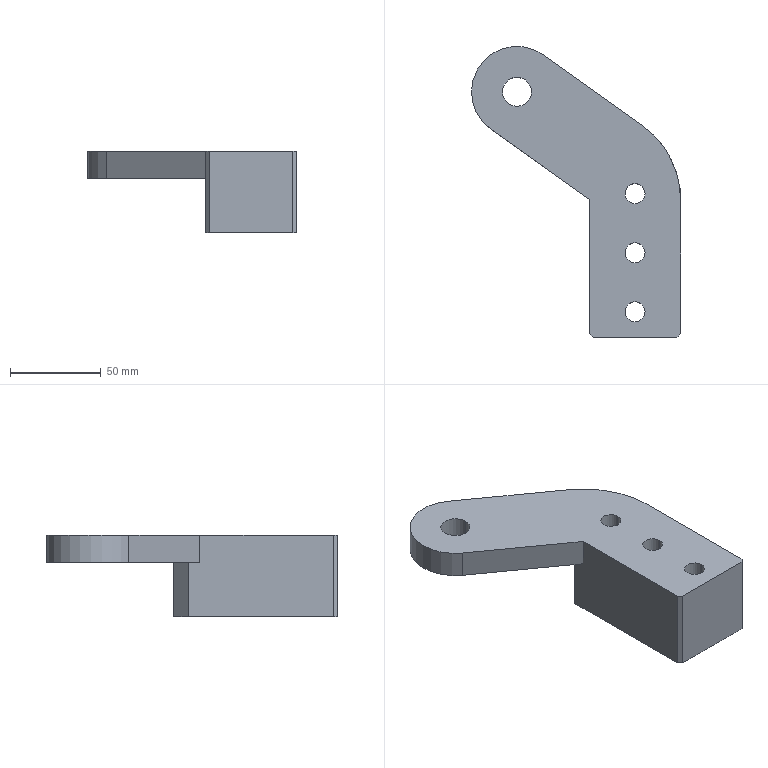Part | Creo | features DATUM PLANE 3, CURVE 2, PROTRUSION 2, CHAMFER 1, COORDINATE SYSTEM 1 | 1 solid | 24 faces | box 115 x 160.005 x 45 mm | volume 256646 mm3 | plane 14 | cylinder 10 | commonest cylinder face diameters 11 x6 16 x2 50 x1 100 x1
STEP:
#1=CARTESIAN_POINT('',(0.,0.,0.));
#2=DIRECTION('',(0.,0.,1.));
#3=DIRECTION('',(1.,0.,0.));
#4=AXIS2_PLACEMENT_3D('',#1,#2,#3);
#5=CARTESIAN_POINT('',(-25.,75.708,0.));
#6=VERTEX_POINT('',#5);
#7=CARTESIAN_POINT('',(-25.,82.,0.));
#8=VERTEX_POINT('',#7);
#9=CARTESIAN_POINT('',(-25.,75.708,0.));
#10=DIRECTION('',(0.,1.,0.));
#11=VECTOR('',#10,6.292);
#12=LINE('',#9,#11);
#13=EDGE_CURVE('',#6,#8,#12,.T.);
#14=ORIENTED_EDGE('',*,*,#13,.T.);
#15=CARTESIAN_POINT('',(-17.,90.,0.));
#16=VERTEX_POINT('',#15);
#17=CARTESIAN_POINT('',(-17.,90.,0.));
#18=DIRECTION('',(-0.7071,-0.7071,0.));
#19=VECTOR('',#18,11.314);
#20=LINE('',#17,#19);
#21=EDGE_CURVE('',#16,#8,#20,.T.);
#22=ORIENTED_EDGE('',*,*,#21,.F.);
#23=CARTESIAN_POINT('',(17.,90.,0.));
#24=VERTEX_POINT('',#23);
#25=CARTESIAN_POINT('',(17.,90.,0.));
#26=DIRECTION('',(-1.,0.,0.));
#27=VECTOR('',#26,34.);
#28=LINE('',#25,#27);
#29=EDGE_CURVE('',#24,#16,#28,.T.);
#30=ORIENTED_EDGE('',*,*,#29,.F.);
#31=CARTESIAN_POINT('',(24.542,82.458,0.));
#32=VERTEX_POINT('',#31);
#33=CARTESIAN_POINT('',(24.542,82.458,0.));
#34=DIRECTION('',(-0.7071,0.7071,0.));
#35=VECTOR('',#34,10.666);
#36=LINE('',#33,#35);
#37=EDGE_CURVE('',#32,#24,#36,.T.);
#38=ORIENTED_EDGE('',*,*,#37,.F.);
#39=CARTESIAN_POINT('',(4.064,116.393,0.));
#40=VERTEX_POINT('',#39);
#41=CARTESIAN_POINT('',(-25.,75.708,0.));
#42=DIRECTION('',(0.,0.,1.));
#43=DIRECTION('',(0.9908,0.135,0.));
#44=AXIS2_PLACEMENT_3D('',#41,#42,#43);
#45=CIRCLE('',#44,50.);
#46=EDGE_CURVE('',#32,#40,#45,.T.);
#47=ORIENTED_EDGE('',*,*,#46,.T.);
#48=CARTESIAN_POINT('',(-50.468,155.348,0.));
#49=VERTEX_POINT('',#48);
#50=CARTESIAN_POINT('',(4.064,116.393,0.));
#51=DIRECTION('',(-0.8137,0.5813,0.));
#52=VECTOR('',#51,67.016);
#53=LINE('',#50,#52);
#54=EDGE_CURVE('',#40,#49,#53,.T.);
#55=ORIENTED_EDGE('',*,*,#54,.T.);
#56=CARTESIAN_POINT('',(-79.532,114.662,0.));
#57=VERTEX_POINT('',#56);
#58=CARTESIAN_POINT('',(-65.,135.005,0.));
#59=DIRECTION('',(0.,0.,1.));
#60=DIRECTION('',(0.5813,0.8137,0.));
#61=AXIS2_PLACEMENT_3D('',#58,#59,#60);
#62=CIRCLE('',#61,25.);
#63=EDGE_CURVE('',#49,#57,#62,.T.);
#64=ORIENTED_EDGE('',*,*,#63,.T.);
#65=CARTESIAN_POINT('',(-79.532,114.662,0.));
#66=DIRECTION('',(0.8137,-0.5813,0.));
#67=VECTOR('',#66,67.016);
#68=LINE('',#65,#67);
#69=EDGE_CURVE('',#57,#6,#68,.T.);
#70=ORIENTED_EDGE('',*,*,#69,.T.);
#71=EDGE_LOOP('',(#14,#22,#30,#38,#47,#55,#64,#70));
#72=FACE_OUTER_BOUND('',#71,.F.);
#73=CARTESIAN_POINT('',(-57.,135.005,0.));
#74=VERTEX_POINT('',#73);
#75=CARTESIAN_POINT('',(-73.,135.005,0.));
#76=VERTEX_POINT('',#75);
#77=CARTESIAN_POINT('',(-65.,135.005,0.));
#78=DIRECTION('',(0.,0.,-1.));
#79=DIRECTION('',(1.,0.,0.));
#80=AXIS2_PLACEMENT_3D('',#77,#78,#79);
#81=CIRCLE('',#80,8.);
#82=EDGE_CURVE('',#74,#76,#81,.T.);
#83=ORIENTED_EDGE('',*,*,#82,.T.);
#84=CARTESIAN_POINT('',(-65.,135.005,0.));
#85=DIRECTION('',(0.,0.,-1.));
#86=DIRECTION('',(-1.,0.,0.));
#87=AXIS2_PLACEMENT_3D('',#84,#85,#86);
#88=CIRCLE('',#87,8.);
#89=EDGE_CURVE('',#76,#74,#88,.T.);
#90=ORIENTED_EDGE('',*,*,#89,.T.);
#91=EDGE_LOOP('',(#83,#90));
#92=FACE_BOUND('',#91,.F.);
#93=CARTESIAN_POINT('',(0.,0.,0.));
#94=DIRECTION('',(0.,0.,1.));
#95=DIRECTION('',(1.,0.,0.));
#96=AXIS2_PLACEMENT_3D('',#93,#94,#95);
#97=PLANE('',#96);
#98=ADVANCED_FACE('',(#72,#92),#97,.F.);
#99=ORIENTED_EDGE('',*,*,#82,.F.);
#100=CARTESIAN_POINT('',(-57.,135.005,15.));
#101=VERTEX_POINT('',#100);
#102=CARTESIAN_POINT('',(-57.,135.005,0.));
#103=DIRECTION('',(0.,0.,1.));
#104=VECTOR('',#103,15.);
#105=LINE('',#102,#104);
#106=EDGE_CURVE('',#74,#101,#105,.T.);
#107=ORIENTED_EDGE('',*,*,#106,.T.);
#108=CARTESIAN_POINT('',(-73.,135.005,15.));
#109=VERTEX_POINT('',#108);
#110=CARTESIAN_POINT('',(-65.,135.005,15.));
#111=DIRECTION('',(0.,0.,-1.));
#112=DIRECTION('',(1.,0.,0.));
#113=AXIS2_PLACEMENT_3D('',#110,#111,#112);
#114=CIRCLE('',#113,8.);
#115=EDGE_CURVE('',#101,#109,#114,.T.);
#116=ORIENTED_EDGE('',*,*,#115,.T.);
#117=CARTESIAN_POINT('',(-73.,135.005,0.));
#118=DIRECTION('',(0.,0.,1.));
#119=VECTOR('',#118,15.);
#120=LINE('',#117,#119);
#121=EDGE_CURVE('',#76,#109,#120,.T.);
#122=ORIENTED_EDGE('',*,*,#121,.F.);
#123=EDGE_LOOP('',(#99,#107,#116,#122));
#124=FACE_OUTER_BOUND('',#123,.F.);
#125=CARTESIAN_POINT('',(-65.,135.005,0.));
#126=DIRECTION('',(0.,0.,1.));
#127=DIRECTION('',(1.,0.,0.));
#128=AXIS2_PLACEMENT_3D('',#125,#126,#127);
#129=CYLINDRICAL_SURFACE('',#128,8.);
#130=ADVANCED_FACE('',(#124),#129,.F.);
#131=ORIENTED_EDGE('',*,*,#89,.F.);
#132=ORIENTED_EDGE('',*,*,#121,.T.);
#133=CARTESIAN_POINT('',(-65.,135.005,15.));
#134=DIRECTION('',(0.,0.,-1.));
#135=DIRECTION('',(-1.,0.,0.));
#136=AXIS2_PLACEMENT_3D('',#133,#134,#135);
#137=CIRCLE('',#136,8.);
#138=EDGE_CURVE('',#109,#101,#137,.T.);
#139=ORIENTED_EDGE('',*,*,#138,.T.);
#140=ORIENTED_EDGE('',*,*,#106,.F.);
#141=EDGE_LOOP('',(#131,#132,#139,#140));
#142=FACE_OUTER_BOUND('',#141,.F.);
#143=CARTESIAN_POINT('',(-65.,135.005,0.));
#144=DIRECTION('',(0.,0.,1.));
#145=DIRECTION('',(1.,0.,0.));
#146=AXIS2_PLACEMENT_3D('',#143,#144,#145);
#147=CYLINDRICAL_SURFACE('',#146,8.);
#148=ADVANCED_FACE('',(#142),#147,.F.);
#149=CARTESIAN_POINT('',(-23.,0.,15.));
#150=VERTEX_POINT('',#149);
#151=CARTESIAN_POINT('',(23.,0.,15.));
#152=VERTEX_POINT('',#151);
#153=CARTESIAN_POINT('',(-23.,0.,15.));
#154=DIRECTION('',(1.,0.,0.));
#155=VECTOR('',#154,46.);
#156=LINE('',#153,#155);
#157=EDGE_CURVE('',#150,#152,#156,.T.);
#158=ORIENTED_EDGE('',*,*,#157,.F.);
#159=CARTESIAN_POINT('',(-25.,2.,15.));
#160=VERTEX_POINT('',#159);
#161=CARTESIAN_POINT('',(-25.,2.,15.));
#162=DIRECTION('',(0.7071,-0.7071,0.));
#163=VECTOR('',#162,2.828);
#164=LINE('',#161,#163);
#165=EDGE_CURVE('',#160,#150,#164,.T.);
#166=ORIENTED_EDGE('',*,*,#165,.F.);
#167=CARTESIAN_POINT('',(-25.,75.708,15.));
#168=VERTEX_POINT('',#167);
#169=CARTESIAN_POINT('',(-25.,75.708,15.));
#170=DIRECTION('',(0.,-1.,0.));
#171=VECTOR('',#170,73.708);
#172=LINE('',#169,#171);
#173=EDGE_CURVE('',#168,#160,#172,.T.);
#174=ORIENTED_EDGE('',*,*,#173,.F.);
#175=CARTESIAN_POINT('',(-79.532,114.662,15.));
#176=VERTEX_POINT('',#175);
#177=CARTESIAN_POINT('',(-79.532,114.662,15.));
#178=DIRECTION('',(0.8137,-0.5813,0.));
#179=VECTOR('',#178,67.016);
#180=LINE('',#177,#179);
#181=EDGE_CURVE('',#176,#168,#180,.T.);
#182=ORIENTED_EDGE('',*,*,#181,.F.);
#183=CARTESIAN_POINT('',(-50.468,155.348,15.));
#184=VERTEX_POINT('',#183);
#185=CARTESIAN_POINT('',(-65.,135.005,15.));
#186=DIRECTION('',(0.,0.,1.));
#187=DIRECTION('',(0.5813,0.8137,0.));
#188=AXIS2_PLACEMENT_3D('',#185,#186,#187);
#189=CIRCLE('',#188,25.);
#190=EDGE_CURVE('',#184,#176,#189,.T.);
#191=ORIENTED_EDGE('',*,*,#190,.F.);
#192=CARTESIAN_POINT('',(4.064,116.393,15.));
#193=VERTEX_POINT('',#192);
#194=CARTESIAN_POINT('',(4.064,116.393,15.));
#195=DIRECTION('',(-0.8137,0.5813,0.));
#196=VECTOR('',#195,67.016);
#197=LINE('',#194,#196);
#198=EDGE_CURVE('',#193,#184,#197,.T.);
#199=ORIENTED_EDGE('',*,*,#198,.F.);
#200=CARTESIAN_POINT('',(25.,75.708,15.));
#201=VERTEX_POINT('',#200);
#202=CARTESIAN_POINT('',(-25.,75.708,15.));
#203=DIRECTION('',(0.,0.,1.));
#204=DIRECTION('',(1.,0.,0.));
#205=AXIS2_PLACEMENT_3D('',#202,#203,#204);
#206=CIRCLE('',#205,50.);
#207=EDGE_CURVE('',#201,#193,#206,.T.);
#208=ORIENTED_EDGE('',*,*,#207,.F.);
#209=CARTESIAN_POINT('',(25.,2.,15.));
#210=VERTEX_POINT('',#209);
#211=CARTESIAN_POINT('',(25.,2.,15.));
#212=DIRECTION('',(0.,1.,0.));
#213=VECTOR('',#212,73.708);
#214=LINE('',#211,#213);
#215=EDGE_CURVE('',#210,#201,#214,.T.);
#216=ORIENTED_EDGE('',*,*,#215,.F.);
#217=CARTESIAN_POINT('',(23.,0.,15.));
#218=DIRECTION('',(0.7071,0.7071,0.));
#219=VECTOR('',#218,2.828);
#220=LINE('',#217,#219);
#221=EDGE_CURVE('',#152,#210,#220,.T.);
#222=ORIENTED_EDGE('',*,*,#221,.F.);
#223=EDGE_LOOP('',(#158,#166,#174,#182,#191,#199,#208,#216,#222));
#224=FACE_OUTER_BOUND('',#223,.F.);
#225=CARTESIAN_POINT('',(5.5,79.,15.));
#226=VERTEX_POINT('',#225);
#227=CARTESIAN_POINT('',(-5.5,79.,15.));
#228=VERTEX_POINT('',#227);
#229=CARTESIAN_POINT('',(0.,79.,15.));
#230=DIRECTION('',(0.,0.,-1.));
#231=DIRECTION('',(1.,0.,0.));
#232=AXIS2_PLACEMENT_3D('',#229,#230,#231);
#233=CIRCLE('',#232,5.5);
#234=EDGE_CURVE('',#226,#228,#233,.T.);
#235=ORIENTED_EDGE('',*,*,#234,.F.);
#236=CARTESIAN_POINT('',(0.,79.,15.));
#237=DIRECTION('',(0.,0.,-1.));
#238=DIRECTION('',(-1.,0.,0.));
#239=AXIS2_PLACEMENT_3D('',#236,#237,#238);
#240=CIRCLE('',#239,5.5);
#241=EDGE_CURVE('',#228,#226,#240,.T.);
#242=ORIENTED_EDGE('',*,*,#241,.F.);
#243=EDGE_LOOP('',(#235,#242));
#244=FACE_BOUND('',#243,.F.);
#245=CARTESIAN_POINT('',(5.5,46.5,15.));
#246=VERTEX_POINT('',#245);
#247=CARTESIAN_POINT('',(-5.5,46.5,15.));
#248=VERTEX_POINT('',#247);
#249=CARTESIAN_POINT('',(0.,46.5,15.));
#250=DIRECTION('',(0.,0.,-1.));
#251=DIRECTION('',(1.,0.,0.));
#252=AXIS2_PLACEMENT_3D('',#249,#250,#251);
#253=CIRCLE('',#252,5.5);
#254=EDGE_CURVE('',#246,#248,#253,.T.);
#255=ORIENTED_EDGE('',*,*,#254,.F.);
#256=CARTESIAN_POINT('',(0.,46.5,15.));
#257=DIRECTION('',(0.,0.,-1.));
#258=DIRECTION('',(-1.,0.,0.));
#259=AXIS2_PLACEMENT_3D('',#256,#257,#258);
#260=CIRCLE('',#259,5.5);
#261=EDGE_CURVE('',#248,#246,#260,.T.);
#262=ORIENTED_EDGE('',*,*,#261,.F.);
#263=EDGE_LOOP('',(#255,#262));
#264=FACE_BOUND('',#263,.F.);
#265=ORIENTED_EDGE('',*,*,#115,.F.);
#266=ORIENTED_EDGE('',*,*,#138,.F.);
#267=EDGE_LOOP('',(#265,#266));
#268=FACE_BOUND('',#267,.F.);
#269=CARTESIAN_POINT('',(5.5,14.,15.));
#270=VERTEX_POINT('',#269);
#271=CARTESIAN_POINT('',(-5.5,14.,15.));
#272=VERTEX_POINT('',#271);
#273=CARTESIAN_POINT('',(0.,14.,15.));
#274=DIRECTION('',(0.,0.,-1.));
#275=DIRECTION('',(1.,0.,0.));
#276=AXIS2_PLACEMENT_3D('',#273,#274,#275);
#277=CIRCLE('',#276,5.5);
#278=EDGE_CURVE('',#270,#272,#277,.T.);
#279=ORIENTED_EDGE('',*,*,#278,.F.);
#280=CARTESIAN_POINT('',(0.,14.,15.));
#281=DIRECTION('',(0.,0.,-1.));
#282=DIRECTION('',(-1.,0.,0.));
#283=AXIS2_PLACEMENT_3D('',#280,#281,#282);
#284=CIRCLE('',#283,5.5);
#285=EDGE_CURVE('',#272,#270,#284,.T.);
#286=ORIENTED_EDGE('',*,*,#285,.F.);
#287=EDGE_LOOP('',(#279,#286));
#288=FACE_BOUND('',#287,.F.);
#289=CARTESIAN_POINT('',(0.,0.,15.));
#290=DIRECTION('',(0.,0.,1.));
#291=DIRECTION('',(1.,0.,0.));
#292=AXIS2_PLACEMENT_3D('',#289,#290,#291);
#293=PLANE('',#292);
#294=ADVANCED_FACE('',(#224,#244,#264,#268,#288),#293,.T.);
#295=CARTESIAN_POINT('',(-5.5,14.,-30.));
#296=VERTEX_POINT('',#295);
#297=CARTESIAN_POINT('',(-5.5,14.,15.));
#298=DIRECTION('',(0.,0.,-1.));
#299=VECTOR('',#298,45.);
#300=LINE('',#297,#299);
#301=EDGE_CURVE('',#272,#296,#300,.T.);
#302=ORIENTED_EDGE('',*,*,#301,.T.);
#303=CARTESIAN_POINT('',(5.5,14.,-30.));
#304=VERTEX_POINT('',#303);
#305=CARTESIAN_POINT('',(0.,14.,-30.));
#306=DIRECTION('',(0.,0.,1.));
#307=DIRECTION('',(-1.,0.,0.));
#308=AXIS2_PLACEMENT_3D('',#305,#306,#307);
#309=CIRCLE('',#308,5.5);
#310=EDGE_CURVE('',#296,#304,#309,.T.);
#311=ORIENTED_EDGE('',*,*,#310,.T.);
#312=CARTESIAN_POINT('',(5.5,14.,-30.));
#313=DIRECTION('',(0.,0.,1.));
#314=VECTOR('',#313,45.);
#315=LINE('',#312,#314);
#316=EDGE_CURVE('',#304,#270,#315,.T.);
#317=ORIENTED_EDGE('',*,*,#316,.T.);
#318=ORIENTED_EDGE('',*,*,#278,.T.);
#319=EDGE_LOOP('',(#302,#311,#317,#318));
#320=FACE_OUTER_BOUND('',#319,.F.);
#321=CARTESIAN_POINT('',(0.,14.,0.));
#322=DIRECTION('',(0.,0.,1.));
#323=DIRECTION('',(1.,0.,0.));
#324=AXIS2_PLACEMENT_3D('',#321,#322,#323);
#325=CYLINDRICAL_SURFACE('',#324,5.5);
#326=ADVANCED_FACE('',(#320),#325,.F.);
#327=ORIENTED_EDGE('',*,*,#316,.F.);
#328=CARTESIAN_POINT('',(0.,14.,-30.));
#329=DIRECTION('',(0.,0.,1.));
#330=DIRECTION('',(1.,0.,0.));
#331=AXIS2_PLACEMENT_3D('',#328,#329,#330);
#332=CIRCLE('',#331,5.5);
#333=EDGE_CURVE('',#304,#296,#332,.T.);
#334=ORIENTED_EDGE('',*,*,#333,.T.);
#335=ORIENTED_EDGE('',*,*,#301,.F.);
#336=ORIENTED_EDGE('',*,*,#285,.T.);
#337=EDGE_LOOP('',(#327,#334,#335,#336));
#338=FACE_OUTER_BOUND('',#337,.F.);
#339=CARTESIAN_POINT('',(0.,14.,0.));
#340=DIRECTION('',(0.,0.,1.));
#341=DIRECTION('',(1.,0.,0.));
#342=AXIS2_PLACEMENT_3D('',#339,#340,#341);
#343=CYLINDRICAL_SURFACE('',#342,5.5);
#344=ADVANCED_FACE('',(#338),#343,.F.);
#345=CARTESIAN_POINT('',(17.,90.,-30.));
#346=VERTEX_POINT('',#345);
#347=CARTESIAN_POINT('',(25.,82.,-30.));
#348=VERTEX_POINT('',#347);
#349=CARTESIAN_POINT('',(17.,90.,-30.));
#350=DIRECTION('',(0.7071,-0.7071,0.));
#351=VECTOR('',#350,11.314);
#352=LINE('',#349,#351);
#353=EDGE_CURVE('',#346,#348,#352,.T.);
#354=ORIENTED_EDGE('',*,*,#353,.F.);
#355=CARTESIAN_POINT('',(-17.,90.,-30.));
#356=VERTEX_POINT('',#355);
#357=CARTESIAN_POINT('',(-17.,90.,-30.));
#358=DIRECTION('',(1.,0.,0.));
#359=VECTOR('',#358,34.);
#360=LINE('',#357,#359);
#361=EDGE_CURVE('',#356,#346,#360,.T.);
#362=ORIENTED_EDGE('',*,*,#361,.F.);
#363=CARTESIAN_POINT('',(-25.,82.,-30.));
#364=VERTEX_POINT('',#363);
#365=CARTESIAN_POINT('',(-25.,82.,-30.));
#366=DIRECTION('',(0.7071,0.7071,0.));
#367=VECTOR('',#366,11.314);
#368=LINE('',#365,#367);
#369=EDGE_CURVE('',#364,#356,#368,.T.);
#370=ORIENTED_EDGE('',*,*,#369,.F.);
#371=CARTESIAN_POINT('',(-25.,2.,-30.));
#372=VERTEX_POINT('',#371);
#373=CARTESIAN_POINT('',(-25.,2.,-30.));
#374=DIRECTION('',(0.,1.,0.));
#375=VECTOR('',#374,80.);
#376=LINE('',#373,#375);
#377=EDGE_CURVE('',#372,#364,#376,.T.);
#378=ORIENTED_EDGE('',*,*,#377,.F.);
#379=CARTESIAN_POINT('',(-23.,0.,-30.));
#380=VERTEX_POINT('',#379);
#381=CARTESIAN_POINT('',(-23.,0.,-30.));
#382=DIRECTION('',(-0.7071,0.7071,0.));
#383=VECTOR('',#382,2.828);
#384=LINE('',#381,#383);
#385=EDGE_CURVE('',#380,#372,#384,.T.);
#386=ORIENTED_EDGE('',*,*,#385,.F.);
#387=CARTESIAN_POINT('',(23.,0.,-30.));
#388=VERTEX_POINT('',#387);
#389=CARTESIAN_POINT('',(23.,0.,-30.));
#390=DIRECTION('',(-1.,0.,0.));
#391=VECTOR('',#390,46.);
#392=LINE('',#389,#391);
#393=EDGE_CURVE('',#388,#380,#392,.T.);
#394=ORIENTED_EDGE('',*,*,#393,.F.);
#395=CARTESIAN_POINT('',(25.,2.,-30.));
#396=VERTEX_POINT('',#395);
#397=CARTESIAN_POINT('',(25.,2.,-30.));
#398=DIRECTION('',(-0.7071,-0.7071,0.));
#399=VECTOR('',#398,2.828);
#400=LINE('',#397,#399);
#401=EDGE_CURVE('',#396,#388,#400,.T.);
#402=ORIENTED_EDGE('',*,*,#401,.F.);
#403=CARTESIAN_POINT('',(25.,82.,-30.));
#404=DIRECTION('',(0.,-1.,0.));
#405=VECTOR('',#404,80.);
#406=LINE('',#403,#405);
#407=EDGE_CURVE('',#348,#396,#406,.T.);
#408=ORIENTED_EDGE('',*,*,#407,.F.);
#409=EDGE_LOOP('',(#354,#362,#370,#378,#386,#394,#402,#408));
#410=FACE_OUTER_BOUND('',#409,.F.);
#411=CARTESIAN_POINT('',(-5.5,46.5,-30.));
#412=VERTEX_POINT('',#411);
#413=CARTESIAN_POINT('',(5.5,46.5,-30.));
#414=VERTEX_POINT('',#413);
#415=CARTESIAN_POINT('',(0.,46.5,-30.));
#416=DIRECTION('',(0.,0.,1.));
#417=DIRECTION('',(-1.,0.,0.));
#418=AXIS2_PLACEMENT_3D('',#415,#416,#417);
#419=CIRCLE('',#418,5.5);
#420=EDGE_CURVE('',#412,#414,#419,.T.);
#421=ORIENTED_EDGE('',*,*,#420,.F.);
#422=CARTESIAN_POINT('',(0.,46.5,-30.));
#423=DIRECTION('',(0.,0.,1.));
#424=DIRECTION('',(1.,0.,0.));
#425=AXIS2_PLACEMENT_3D('',#422,#423,#424);
#426=CIRCLE('',#425,5.5);
#427=EDGE_CURVE('',#414,#412,#426,.T.);
#428=ORIENTED_EDGE('',*,*,#427,.F.);
#429=EDGE_LOOP('',(#421,#428));
#430=FACE_BOUND('',#429,.F.);
#431=ORIENTED_EDGE('',*,*,#333,.F.);
#432=ORIENTED_EDGE('',*,*,#310,.F.);
#433=EDGE_LOOP('',(#431,#432));
#434=FACE_BOUND('',#433,.F.);
#435=CARTESIAN_POINT('',(-5.5,79.,-30.));
#436=VERTEX_POINT('',#435);
#437=CARTESIAN_POINT('',(5.5,79.,-30.));
#438=VERTEX_POINT('',#437);
#439=CARTESIAN_POINT('',(0.,79.,-30.));
#440=DIRECTION('',(0.,0.,1.));
#441=DIRECTION('',(-1.,0.,0.));
#442=AXIS2_PLACEMENT_3D('',#439,#440,#441);
#443=CIRCLE('',#442,5.5);
#444=EDGE_CURVE('',#436,#438,#443,.T.);
#445=ORIENTED_EDGE('',*,*,#444,.F.);
#446=CARTESIAN_POINT('',(0.,79.,-30.));
#447=DIRECTION('',(0.,0.,1.));
#448=DIRECTION('',(1.,0.,0.));
#449=AXIS2_PLACEMENT_3D('',#446,#447,#448);
#450=CIRCLE('',#449,5.5);
#451=EDGE_CURVE('',#438,#436,#450,.T.);
#452=ORIENTED_EDGE('',*,*,#451,.F.);
#453=EDGE_LOOP('',(#445,#452));
#454=FACE_BOUND('',#453,.F.);
#455=CARTESIAN_POINT('',(0.,0.,-30.));
#456=DIRECTION('',(0.,0.,-1.));
#457=DIRECTION('',(-1.,0.,0.));
#458=AXIS2_PLACEMENT_3D('',#455,#456,#457);
#459=PLANE('',#458);
#460=ADVANCED_FACE('',(#410,#430,#434,#454),#459,.T.);
#461=CARTESIAN_POINT('',(-5.5,79.,-30.));
#462=DIRECTION('',(0.,0.,1.));
#463=VECTOR('',#462,45.);
#464=LINE('',#461,#463);
#465=EDGE_CURVE('',#436,#228,#464,.T.);
#466=ORIENTED_EDGE('',*,*,#465,.F.);
#467=ORIENTED_EDGE('',*,*,#444,.T.);
#468=CARTESIAN_POINT('',(5.5,79.,15.));
#469=DIRECTION('',(0.,0.,-1.));
#470=VECTOR('',#469,45.);
#471=LINE('',#468,#470);
#472=EDGE_CURVE('',#226,#438,#471,.T.);
#473=ORIENTED_EDGE('',*,*,#472,.F.);
#474=ORIENTED_EDGE('',*,*,#234,.T.);
#475=EDGE_LOOP('',(#466,#467,#473,#474));
#476=FACE_OUTER_BOUND('',#475,.F.);
#477=CARTESIAN_POINT('',(0.,79.,0.));
#478=DIRECTION('',(0.,0.,1.));
#479=DIRECTION('',(1.,0.,0.));
#480=AXIS2_PLACEMENT_3D('',#477,#478,#479);
#481=CYLINDRICAL_SURFACE('',#480,5.5);
#482=ADVANCED_FACE('',(#476),#481,.F.);
#483=ORIENTED_EDGE('',*,*,#472,.T.);
#484=ORIENTED_EDGE('',*,*,#451,.T.);
#485=ORIENTED_EDGE('',*,*,#465,.T.);
#486=ORIENTED_EDGE('',*,*,#241,.T.);
#487=EDGE_LOOP('',(#483,#484,#485,#486));
#488=FACE_OUTER_BOUND('',#487,.F.);
#489=CARTESIAN_POINT('',(0.,79.,0.));
#490=DIRECTION('',(0.,0.,1.));
#491=DIRECTION('',(1.,0.,0.));
#492=AXIS2_PLACEMENT_3D('',#489,#490,#491);
#493=CYLINDRICAL_SURFACE('',#492,5.5);
#494=ADVANCED_FACE('',(#488),#493,.F.);
#495=CARTESIAN_POINT('',(-5.5,46.5,-30.));
#496=DIRECTION('',(0.,0.,1.));
#497=VECTOR('',#496,45.);
#498=LINE('',#495,#497);
#499=EDGE_CURVE('',#412,#248,#498,.T.);
#500=ORIENTED_EDGE('',*,*,#499,.F.);
#501=ORIENTED_EDGE('',*,*,#420,.T.);
#502=CARTESIAN_POINT('',(5.5,46.5,15.));
#503=DIRECTION('',(0.,0.,-1.));
#504=VECTOR('',#503,45.);
#505=LINE('',#502,#504);
#506=EDGE_CURVE('',#246,#414,#505,.T.);
#507=ORIENTED_EDGE('',*,*,#506,.F.);
#508=ORIENTED_EDGE('',*,*,#254,.T.);
#509=EDGE_LOOP('',(#500,#501,#507,#508));
#510=FACE_OUTER_BOUND('',#509,.F.);
#511=CARTESIAN_POINT('',(0.,46.5,0.));
#512=DIRECTION('',(0.,0.,1.));
#513=DIRECTION('',(1.,0.,0.));
#514=AXIS2_PLACEMENT_3D('',#511,#512,#513);
#515=CYLINDRICAL_SURFACE('',#514,5.5);
#516=ADVANCED_FACE('',(#510),#515,.F.);
#517=ORIENTED_EDGE('',*,*,#506,.T.);
#518=ORIENTED_EDGE('',*,*,#427,.T.);
#519=ORIENTED_EDGE('',*,*,#499,.T.);
#520=ORIENTED_EDGE('',*,*,#261,.T.);
#521=EDGE_LOOP('',(#517,#518,#519,#520));
#522=FACE_OUTER_BOUND('',#521,.F.);
#523=CARTESIAN_POINT('',(0.,46.5,0.));
#524=DIRECTION('',(0.,0.,1.));
#525=DIRECTION('',(1.,0.,0.));
#526=AXIS2_PLACEMENT_3D('',#523,#524,#525);
#527=CYLINDRICAL_SURFACE('',#526,5.5);
#528=ADVANCED_FACE('',(#522),#527,.F.);
#529=CARTESIAN_POINT('',(25.,82.,0.));
#530=VERTEX_POINT('',#529);
#531=CARTESIAN_POINT('',(25.,82.,0.));
#532=DIRECTION('',(-0.7071,0.7071,0.));
#533=VECTOR('',#532,0.6473);
#534=LINE('',#531,#533);
#535=EDGE_CURVE('',#530,#32,#534,.T.);
#536=ORIENTED_EDGE('',*,*,#535,.T.);
#537=ORIENTED_EDGE('',*,*,#37,.T.);
#538=CARTESIAN_POINT('',(17.,90.,-30.));
#539=DIRECTION('',(0.,0.,1.));
#540=VECTOR('',#539,30.);
#541=LINE('',#538,#540);
#542=EDGE_CURVE('',#346,#24,#541,.T.);
#543=ORIENTED_EDGE('',*,*,#542,.F.);
#544=ORIENTED_EDGE('',*,*,#353,.T.);
#545=CARTESIAN_POINT('',(25.,82.,-30.));
#546=DIRECTION('',(0.,0.,1.));
#547=VECTOR('',#546,30.);
#548=LINE('',#545,#547);
#549=EDGE_CURVE('',#348,#530,#548,.T.);
#550=ORIENTED_EDGE('',*,*,#549,.T.);
#551=EDGE_LOOP('',(#536,#537,#543,#544,#550));
#552=FACE_OUTER_BOUND('',#551,.F.);
#553=CARTESIAN_POINT('',(21.,86.,-15.));
#554=DIRECTION('',(0.7071,0.7071,0.));
#555=DIRECTION('',(-0.7071,0.7071,0.));
#556=AXIS2_PLACEMENT_3D('',#553,#554,#555);
#557=PLANE('',#556);
#558=ADVANCED_FACE('',(#552),#557,.T.);
#559=ORIENTED_EDGE('',*,*,#535,.F.);
#560=CARTESIAN_POINT('',(25.,75.708,0.));
#561=VERTEX_POINT('',#560);
#562=CARTESIAN_POINT('',(25.,82.,0.));
#563=DIRECTION('',(0.,-1.,0.));
#564=VECTOR('',#563,6.292);
#565=LINE('',#562,#564);
#566=EDGE_CURVE('',#530,#561,#565,.T.);
#567=ORIENTED_EDGE('',*,*,#566,.T.);
#568=CARTESIAN_POINT('',(-25.,75.708,0.));
#569=DIRECTION('',(0.,0.,1.));
#570=DIRECTION('',(1.,0.,0.));
#571=AXIS2_PLACEMENT_3D('',#568,#569,#570);
#572=CIRCLE('',#571,50.);
#573=EDGE_CURVE('',#561,#32,#572,.T.);
#574=ORIENTED_EDGE('',*,*,#573,.T.);
#575=EDGE_LOOP('',(#559,#567,#574));
#576=FACE_OUTER_BOUND('',#575,.F.);
#577=CARTESIAN_POINT('',(0.,0.,0.));
#578=DIRECTION('',(0.,0.,-1.));
#579=DIRECTION('',(-1.,0.,0.));
#580=AXIS2_PLACEMENT_3D('',#577,#578,#579);
#581=PLANE('',#580);
#582=ADVANCED_FACE('',(#576),#581,.F.);
#583=ORIENTED_EDGE('',*,*,#549,.F.);
#584=ORIENTED_EDGE('',*,*,#407,.T.);
#585=CARTESIAN_POINT('',(25.,2.,15.));
#586=DIRECTION('',(0.,0.,-1.));
#587=VECTOR('',#586,45.);
#588=LINE('',#585,#587);
#589=EDGE_CURVE('',#210,#396,#588,.T.);
#590=ORIENTED_EDGE('',*,*,#589,.F.);
#591=ORIENTED_EDGE('',*,*,#215,.T.);
#592=CARTESIAN_POINT('',(25.,75.708,0.));
#593=DIRECTION('',(0.,0.,1.));
#594=VECTOR('',#593,15.);
#595=LINE('',#592,#594);
#596=EDGE_CURVE('',#561,#201,#595,.T.);
#597=ORIENTED_EDGE('',*,*,#596,.F.);
#598=ORIENTED_EDGE('',*,*,#566,.F.);
#599=EDGE_LOOP('',(#583,#584,#590,#591,#597,#598));
#600=FACE_OUTER_BOUND('',#599,.F.);
#601=CARTESIAN_POINT('',(25.,2.,0.));
#602=DIRECTION('',(1.,0.,0.));
#603=DIRECTION('',(0.,1.,0.));
#604=AXIS2_PLACEMENT_3D('',#601,#602,#603);
#605=PLANE('',#604);
#606=ADVANCED_FACE('',(#600),#605,.T.);
#607=ORIENTED_EDGE('',*,*,#589,.T.);
#608=ORIENTED_EDGE('',*,*,#401,.T.);
#609=CARTESIAN_POINT('',(23.,0.,-30.));
#610=DIRECTION('',(0.,0.,1.));
#611=VECTOR('',#610,45.);
#612=LINE('',#609,#611);
#613=EDGE_CURVE('',#388,#152,#612,.T.);
#614=ORIENTED_EDGE('',*,*,#613,.T.);
#615=ORIENTED_EDGE('',*,*,#221,.T.);
#616=EDGE_LOOP('',(#607,#608,#614,#615));
#617=FACE_OUTER_BOUND('',#616,.F.);
#618=CARTESIAN_POINT('',(23.,0.,0.));
#619=DIRECTION('',(0.7071,-0.7071,0.));
#620=DIRECTION('',(0.7071,0.7071,0.));
#621=AXIS2_PLACEMENT_3D('',#618,#619,#620);
#622=PLANE('',#621);
#623=ADVANCED_FACE('',(#617),#622,.T.);
#624=ORIENTED_EDGE('',*,*,#613,.F.);
#625=ORIENTED_EDGE('',*,*,#393,.T.);
#626=CARTESIAN_POINT('',(-23.,0.,15.));
#627=DIRECTION('',(0.,0.,-1.));
#628=VECTOR('',#627,45.);
#629=LINE('',#626,#628);
#630=EDGE_CURVE('',#150,#380,#629,.T.);
#631=ORIENTED_EDGE('',*,*,#630,.F.);
#632=ORIENTED_EDGE('',*,*,#157,.T.);
#633=EDGE_LOOP('',(#624,#625,#631,#632));
#634=FACE_OUTER_BOUND('',#633,.F.);
#635=CARTESIAN_POINT('',(-23.,0.,0.));
#636=DIRECTION('',(0.,-1.,0.));
#637=DIRECTION('',(1.,0.,0.));
#638=AXIS2_PLACEMENT_3D('',#635,#636,#637);
#639=PLANE('',#638);
#640=ADVANCED_FACE('',(#634),#639,.T.);
#641=ORIENTED_EDGE('',*,*,#630,.T.);
#642=ORIENTED_EDGE('',*,*,#385,.T.);
#643=CARTESIAN_POINT('',(-25.,2.,15.));
#644=DIRECTION('',(0.,0.,-1.));
#645=VECTOR('',#644,45.);
#646=LINE('',#643,#645);
#647=EDGE_CURVE('',#160,#372,#646,.T.);
#648=ORIENTED_EDGE('',*,*,#647,.F.);
#649=ORIENTED_EDGE('',*,*,#165,.T.);
#650=EDGE_LOOP('',(#641,#642,#648,#649));
#651=FACE_OUTER_BOUND('',#650,.F.);
#652=CARTESIAN_POINT('',(-25.,2.,0.));
#653=DIRECTION('',(-0.7071,-0.7071,0.));
#654=DIRECTION('',(0.7071,-0.7071,0.));
#655=AXIS2_PLACEMENT_3D('',#652,#653,#654);
#656=PLANE('',#655);
#657=ADVANCED_FACE('',(#651),#656,.T.);
#658=CARTESIAN_POINT('',(-25.,82.,-30.));
#659=DIRECTION('',(0.,0.,1.));
#660=VECTOR('',#659,30.);
#661=LINE('',#658,#660);
#662=EDGE_CURVE('',#364,#8,#661,.T.);
#663=ORIENTED_EDGE('',*,*,#662,.T.);
#664=ORIENTED_EDGE('',*,*,#13,.F.);
#665=CARTESIAN_POINT('',(-25.,75.708,0.));
#666=DIRECTION('',(0.,0.,1.));
#667=VECTOR('',#666,15.);
#668=LINE('',#665,#667);
#669=EDGE_CURVE('',#6,#168,#668,.T.);
#670=ORIENTED_EDGE('',*,*,#669,.T.);
#671=ORIENTED_EDGE('',*,*,#173,.T.);
#672=ORIENTED_EDGE('',*,*,#647,.T.);
#673=ORIENTED_EDGE('',*,*,#377,.T.);
#674=EDGE_LOOP('',(#663,#664,#670,#671,#672,#673));
#675=FACE_OUTER_BOUND('',#674,.F.);
#676=CARTESIAN_POINT('',(-25.,75.708,0.));
#677=DIRECTION('',(-1.,0.,0.));
#678=DIRECTION('',(0.,-1.,0.));
#679=AXIS2_PLACEMENT_3D('',#676,#677,#678);
#680=PLANE('',#679);
#681=ADVANCED_FACE('',(#675),#680,.T.);
#682=ORIENTED_EDGE('',*,*,#662,.F.);
#683=ORIENTED_EDGE('',*,*,#369,.T.);
#684=CARTESIAN_POINT('',(-17.,90.,-30.));
#685=DIRECTION('',(0.,0.,1.));
#686=VECTOR('',#685,30.);
#687=LINE('',#684,#686);
#688=EDGE_CURVE('',#356,#16,#687,.T.);
#689=ORIENTED_EDGE('',*,*,#688,.T.);
#690=ORIENTED_EDGE('',*,*,#21,.T.);
#691=EDGE_LOOP('',(#682,#683,#689,#690));
#692=FACE_OUTER_BOUND('',#691,.F.);
#693=CARTESIAN_POINT('',(-21.,86.,-15.));
#694=DIRECTION('',(-0.7071,0.7071,0.));
#695=DIRECTION('',(-0.7071,-0.7071,0.));
#696=AXIS2_PLACEMENT_3D('',#693,#694,#695);
#697=PLANE('',#696);
#698=ADVANCED_FACE('',(#692),#697,.T.);
#699=ORIENTED_EDGE('',*,*,#542,.T.);
#700=ORIENTED_EDGE('',*,*,#29,.T.);
#701=ORIENTED_EDGE('',*,*,#688,.F.);
#702=ORIENTED_EDGE('',*,*,#361,.T.);
#703=EDGE_LOOP('',(#699,#700,#701,#702));
#704=FACE_OUTER_BOUND('',#703,.F.);
#705=CARTESIAN_POINT('',(-25.,90.,0.));
#706=DIRECTION('',(0.,1.,0.));
#707=DIRECTION('',(1.,0.,0.));
#708=AXIS2_PLACEMENT_3D('',#705,#706,#707);
#709=PLANE('',#708);
#710=ADVANCED_FACE('',(#704),#709,.T.);
#711=ORIENTED_EDGE('',*,*,#69,.F.);
#712=CARTESIAN_POINT('',(-79.532,114.662,0.));
#713=DIRECTION('',(0.,0.,1.));
#714=VECTOR('',#713,15.);
#715=LINE('',#712,#714);
#716=EDGE_CURVE('',#57,#176,#715,.T.);
#717=ORIENTED_EDGE('',*,*,#716,.T.);
#718=ORIENTED_EDGE('',*,*,#181,.T.);
#719=ORIENTED_EDGE('',*,*,#669,.F.);
#720=EDGE_LOOP('',(#711,#717,#718,#719));
#721=FACE_OUTER_BOUND('',#720,.F.);
#722=CARTESIAN_POINT('',(-79.532,114.662,0.));
#723=DIRECTION('',(-0.5813,-0.8137,0.));
#724=DIRECTION('',(0.8137,-0.5813,0.));
#725=AXIS2_PLACEMENT_3D('',#722,#723,#724);
#726=PLANE('',#725);
#727=ADVANCED_FACE('',(#721),#726,.T.);
#728=ORIENTED_EDGE('',*,*,#63,.F.);
#729=CARTESIAN_POINT('',(-50.468,155.348,0.));
#730=DIRECTION('',(0.,0.,1.));
#731=VECTOR('',#730,15.);
#732=LINE('',#729,#731);
#733=EDGE_CURVE('',#49,#184,#732,.T.);
#734=ORIENTED_EDGE('',*,*,#733,.T.);
#735=ORIENTED_EDGE('',*,*,#190,.T.);
#736=ORIENTED_EDGE('',*,*,#716,.F.);
#737=EDGE_LOOP('',(#728,#734,#735,#736));
#738=FACE_OUTER_BOUND('',#737,.F.);
#739=CARTESIAN_POINT('',(-65.,135.005,0.));
#740=DIRECTION('',(0.,0.,1.));
#741=DIRECTION('',(1.,0.,0.));
#742=AXIS2_PLACEMENT_3D('',#739,#740,#741);
#743=CYLINDRICAL_SURFACE('',#742,25.);
#744=ADVANCED_FACE('',(#738),#743,.T.);
#745=ORIENTED_EDGE('',*,*,#54,.F.);
#746=CARTESIAN_POINT('',(4.064,116.393,0.));
#747=DIRECTION('',(0.,0.,1.));
#748=VECTOR('',#747,15.);
#749=LINE('',#746,#748);
#750=EDGE_CURVE('',#40,#193,#749,.T.);
#751=ORIENTED_EDGE('',*,*,#750,.T.);
#752=ORIENTED_EDGE('',*,*,#198,.T.);
#753=ORIENTED_EDGE('',*,*,#733,.F.);
#754=EDGE_LOOP('',(#745,#751,#752,#753));
#755=FACE_OUTER_BOUND('',#754,.F.);
#756=CARTESIAN_POINT('',(4.064,116.393,0.));
#757=DIRECTION('',(0.5813,0.8137,0.));
#758=DIRECTION('',(-0.8137,0.5813,0.));
#759=AXIS2_PLACEMENT_3D('',#756,#757,#758);
#760=PLANE('',#759);
#761=ADVANCED_FACE('',(#755),#760,.T.);
#762=ORIENTED_EDGE('',*,*,#46,.F.);
#763=ORIENTED_EDGE('',*,*,#573,.F.);
#764=ORIENTED_EDGE('',*,*,#596,.T.);
#765=ORIENTED_EDGE('',*,*,#207,.T.);
#766=ORIENTED_EDGE('',*,*,#750,.F.);
#767=EDGE_LOOP('',(#762,#763,#764,#765,#766));
#768=FACE_OUTER_BOUND('',#767,.F.);
#769=CARTESIAN_POINT('',(-25.,75.708,0.));
#770=DIRECTION('',(0.,0.,1.));
#771=DIRECTION('',(1.,0.,0.));
#772=AXIS2_PLACEMENT_3D('',#769,#770,#771);
#773=CYLINDRICAL_SURFACE('',#772,50.);
#774=ADVANCED_FACE('',(#768),#773,.T.);
#775=CLOSED_SHELL('',(#98,#130,#148,#294,#326,#344,#460,#482,#494,#516,#528,#558,#582,#606,#623,#640,#657,#681,#698,#710,#727,#744,#761,#774));
#776=MANIFOLD_SOLID_BREP('',#775);
#777=(LENGTH_UNIT()NAMED_UNIT(*)SI_UNIT(.MILLI.,.METRE.));
#778=UNCERTAINTY_MEASURE_WITH_UNIT(LENGTH_MEASURE(0.02021),#777,'','');
#779=(NAMED_UNIT(*)PLANE_ANGLE_UNIT()SI_UNIT($,.RADIAN.));
#780=PLANE_ANGLE_MEASURE_WITH_UNIT(PLANE_ANGLE_MEASURE(0.01745),#779);
#781=(CONVERSION_BASED_UNIT('DEGREE',#780)NAMED_UNIT(*)PLANE_ANGLE_UNIT());
#782=(NAMED_UNIT(*)SI_UNIT($,.STERADIAN.)SOLID_ANGLE_UNIT());
#783=(GEOMETRIC_REPRESENTATION_CONTEXT(3)GLOBAL_UNCERTAINTY_ASSIGNED_CONTEXT((#778))GLOBAL_UNIT_ASSIGNED_CONTEXT((#777,#781,#782))REPRESENTATION_CONTEXT('',''));
#784=ADVANCED_BREP_SHAPE_REPRESENTATION('',(#4,#776),#783);